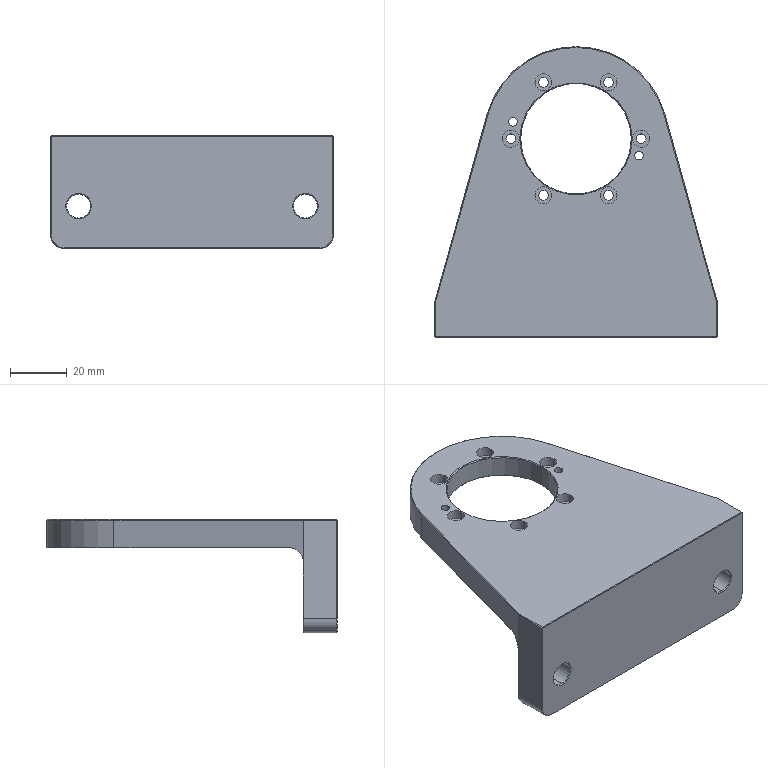NC program | NX | posted with a generic post | part box 100 x 102.5 x 40 mm
Lines 4148 to 4503 of 4503:
(ZLEVEL_PROFILE_COPY_1_COPY_COPY_1 , TOOL : D10JING)
N8264 T14 M6
N8266 G54
N8268 G17 G0 G90 X-58.059 Y-51.322 B0. C0. S9500 M3
N8270 G43 Z30. H14
N8272 Z-19.
N8274 G94 G1 Z-20. F1000.
N8276 X-56.75 Y-50.566
N8278 G3 X-56.25 Y-49.7 R1.
N8280 G1 Y49.7 F1200.
N8282 G2 X-54.786 Y53.236 R5.
N8284 G1 X-54.486 Y53.536
N8286 G2 X-50.95 Y55. R5.
N8288 G1 X-39.25
N8290 G2 X-37.901 Y54.815 R5.
N8292 G1 X28.866 Y36.11
N8294 G2 X28.866 Y-36.11 R37.5
N8296 G1 X-37.901 Y-54.815
N8298 G2 X-39.25 Y-55. R5.
N8300 G1 X-50.95
N8302 G2 X-54.486 Y-53.536 R5.
N8304 G1 X-54.786 Y-53.236
N8306 G2 X-56.25 Y-49.7 R5.
N8308 G3 X-56.75 Y-48.834 R1.
N8310 G1 X-58.25 Y-47.968
N8312 Z-19.
N8314 G0 Z30.
N8316 X-58.059 Y-51.322
N8318 Z-39.
N8320 G1 Z-40. F1000.
N8322 X-56.75 Y-50.566
N8324 G3 X-56.25 Y-49.7 R1.
N8326 G1 Y49.7 F1200.
N8328 G2 X-54.786 Y53.236 R5.
N8330 G1 X-54.486 Y53.536
N8332 G2 X-50.95 Y55. R5.
N8334 G1 X-39.25
N8336 G2 X-37.901 Y54.815 R5.
N8338 G1 X28.866 Y36.11
N8340 G2 X28.866 Y-36.11 R37.5
N8342 G1 X-37.901 Y-54.815
N8344 G2 X-39.25 Y-55. R5.
N8346 G1 X-50.95
N8348 G2 X-54.486 Y-53.536 R5.
N8350 G1 X-54.786 Y-53.236
N8352 G2 X-56.25 Y-49.7 R5.
N8354 G3 X-56.75 Y-48.834 R1.
N8356 G1 X-58.25 Y-47.968
N8358 Z-39.
N8360 G0 Z30.
(ZLEVEL_PROFILE_COPY_1_COPY_COPY_1_COPY , TOOL : D10JING)
N8362 X31.119 Y-1.808
N8364 Z-9.
N8366 G1 Z-10. F1000.
N8368 X32.75 Y-0.866
N8370 G3 X33.25 Y0. R1.
N8372 X18.75 Y14.5 R14.5 F1200.
N8374 X33.25 Y0. R-14.5
N8376 X32.75 Y0.866 R1.
N8378 G1 X31.119 Y1.808
N8380 Z-9.
N8382 G0 Z30.
N8384 M5
(HOLE_MILLING_1 , TOOL : D4)
N8386 T11 M6
N8388 G54
N8390 G17 G0 G90 X-1.169 Y11.5 B0. C0. S9500 M3
N8392 G43 Z30. H11
N8394 Z0.5
N8396 G94 G3 X-1.669 Y11. R0.5 F1350.
N8398 X-1.169 Y10.5 R0.5
N8400 X-1.169 Y10.5 Z0.15 I0. J1.
N8402 X-1.169 Y10.5 Z-0.2 I0. J1.
N8404 X-1.169 Y10.5 Z-0.55 I0. J1.
N8406 X-1.169 Y10.5 Z-0.9 I0. J1.
N8408 X-1.169 Y10.5 Z-1.25 I0. J1.
N8410 X-1.169 Y10.5 Z-1.6 I0. J1.
N8412 X-1.169 Y10.5 Z-1.95 I0. J1.
N8414 X-1.169 Y10.5 Z-2.3 I0. J1.
N8416 X-1.169 Y10.5 Z-2.65 I0. J1.
N8418 X-1.169 Y10.5 Z-3. I0. J1.
N8420 X-1.169 Y10.5 Z-3.35 I0. J1.
N8422 X-0.387 Y10.877 Z-3.4 R1.
N8424 X-0.545 Y12.282 R1.
N8426 X-0.387 Y10.877 R-1.
N8428 X-0.466 Y11.579 R0.5
N8430 X-1.169 Y11.5 R0.5
N8432 G0 Z30.
N8434 X18.75 Y23.
N8436 Z0.5
N8438 G3 X18.25 Y22.5 R0.5
N8440 X18.75 Y22. R0.5
N8442 X18.75 Y22. Z0.15 I0. J1.
N8444 X18.75 Y22. Z-0.2 I0. J1.
N8446 X18.75 Y22. Z-0.55 I0. J1.
N8448 X18.75 Y22. Z-0.9 I0. J1.
N8450 X18.75 Y22. Z-1.25 I0. J1.
N8452 X18.75 Y22. Z-1.6 I0. J1.
N8454 X18.75 Y22. Z-1.95 I0. J1.
N8456 X18.75 Y22. Z-2.3 I0. J1.
N8458 X18.75 Y22. Z-2.65 I0. J1.
N8460 X18.75 Y22. Z-3. I0. J1.
N8462 X18.75 Y22. Z-3.35 I0. J1.
N8464 X19.532 Y22.377 Z-3.4 R1.
N8466 X19.373 Y23.782 R1.
N8468 X19.532 Y22.377 R-1.
N8470 X19.453 Y23.079 R0.5
N8472 X18.75 Y23. R0.5
N8474 G0 Z30.
N8476 X38.669 Y11.5
N8478 Z0.5
N8480 G3 X38.169 Y11. R0.5
N8482 X38.669 Y10.5 R0.5
N8484 X38.669 Y10.5 Z0.15 I0. J1.
N8486 X38.669 Y10.5 Z-0.2 I0. J1.
N8488 X38.669 Y10.5 Z-0.55 I0. J1.
N8490 X38.669 Y10.5 Z-0.9 I0. J1.
N8492 X38.669 Y10.5 Z-1.25 I0. J1.
N8494 X38.669 Y10.5 Z-1.6 I0. J1.
N8496 X38.669 Y10.5 Z-1.95 I0. J1.
N8498 X38.669 Y10.5 Z-2.3 I0. J1.
N8500 X38.669 Y10.5 Z-2.65 I0. J1.
N8502 X38.669 Y10.5 Z-3. I0. J1.
N8504 X38.669 Y10.5 Z-3.35 I0. J1.
N8506 X39.45 Y10.877 Z-3.4 R1.
N8508 X39.292 Y12.282 R1.
N8510 X39.45 Y10.877 R-1.
N8512 X39.371 Y11.579 R0.5
N8514 X38.669 Y11.5 R0.5
N8516 G0 Z30.
N8518 Y-11.5
N8520 Z0.5
N8522 G3 X38.169 Y-12. R0.5
N8524 X38.669 Y-12.5 R0.5
N8526 X38.669 Y-12.5 Z0.15 I0. J1.
N8528 X38.669 Y-12.5 Z-0.2 I0. J1.
N8530 X38.669 Y-12.5 Z-0.55 I0. J1.
N8532 X38.669 Y-12.5 Z-0.9 I0. J1.
N8534 X38.669 Y-12.5 Z-1.25 I0. J1.
N8536 X38.669 Y-12.5 Z-1.6 I0. J1.
N8538 X38.669 Y-12.5 Z-1.95 I0. J1.
N8540 X38.669 Y-12.5 Z-2.3 I0. J1.
N8542 X38.669 Y-12.5 Z-2.65 I0. J1.
N8544 X38.669 Y-12.5 Z-3. I0. J1.
N8546 X38.669 Y-12.5 Z-3.35 I0. J1.
N8548 X39.45 Y-12.123 Z-3.4 R1.
N8550 X39.292 Y-10.718 R1.
N8552 X39.45 Y-12.123 R-1.
N8554 X39.371 Y-11.421 R0.5
N8556 X38.669 Y-11.5 R0.5
N8558 G0 Z30.
N8560 X18.75 Y-23.
N8562 Z0.5
N8564 G3 X18.25 Y-23.5 R0.5
N8566 X18.75 Y-24. R0.5
N8568 X18.75 Y-24. Z0.15 I0. J1.
N8570 X18.75 Y-24. Z-0.2 I0. J1.
N8572 X18.75 Y-24. Z-0.55 I0. J1.
N8574 X18.75 Y-24. Z-0.9 I0. J1.
N8576 X18.75 Y-24. Z-1.25 I0. J1.
N8578 X18.75 Y-24. Z-1.6 I0. J1.
N8580 X18.75 Y-24. Z-1.95 I0. J1.
N8582 X18.75 Y-24. Z-2.3 I0. J1.
N8584 X18.75 Y-24. Z-2.65 I0. J1.
N8586 X18.75 Y-24. Z-3. I0. J1.
N8588 X18.75 Y-24. Z-3.35 I0. J1.
N8590 X19.532 Y-23.623 Z-3.4 R1.
N8592 X19.373 Y-22.218 R1.
N8594 X19.532 Y-23.623 R-1.
N8596 X19.453 Y-22.921 R0.5
N8598 X18.75 Y-23. R0.5
N8600 G0 Z30.
N8602 X-1.169 Y-11.5
N8604 Z0.5
N8606 G3 X-1.669 Y-12. R0.5
N8608 X-1.169 Y-12.5 R0.5
N8610 X-1.169 Y-12.5 Z0.15 I0. J1.
N8612 X-1.169 Y-12.5 Z-0.2 I0. J1.
N8614 X-1.169 Y-12.5 Z-0.55 I0. J1.
N8616 X-1.169 Y-12.5 Z-0.9 I0. J1.
N8618 X-1.169 Y-12.5 Z-1.25 I0. J1.
N8620 X-1.169 Y-12.5 Z-1.6 I0. J1.
N8622 X-1.169 Y-12.5 Z-1.95 I0. J1.
N8624 X-1.169 Y-12.5 Z-2.3 I0. J1.
N8626 X-1.169 Y-12.5 Z-2.65 I0. J1.
N8628 X-1.169 Y-12.5 Z-3. I0. J1.
N8630 X-1.169 Y-12.5 Z-3.35 I0. J1.
N8632 X-0.387 Y-12.123 Z-3.4 R1.
N8634 X-0.545 Y-10.718 R1.
N8636 X-0.387 Y-12.123 R-1.
N8638 X-0.466 Y-11.421 R0.5
N8640 X-1.169 Y-11.5 R0.5
N8642 G0 Z30.
N8644 M5
(PLANAR_MILL_COPY_COPY_COPY_COPY_COPY_COPY_1_COPY_1 , TOOL : D6A45)
N8646 T01 M6
N8648 G54
N8650 G17 G0 G90 X19.616 Y24.7 B0. C0. S9500 M3
N8652 G43 Z30. H1
N8654 Z0.5
N8656 G94 G1 Z-1. F1250.
N8658 G3 X18.75 Y25.2 R1.
N8660 X16.55 Y23. R2.2
N8662 X18.75 Y25.2 R-2.2
N8664 X17.884 Y24.7 R1.
N8666 G1 Z0.5
N8668 G0 Z30.
N8670 X25.153 Y21.783
N8672 Z0.5
N8674 G1 Z-1.
N8676 G3 X25.403 Y22.216 R0.5
N8678 X24.703 Y22.916 R0.7
N8680 X25.403 Y22.216 R-0.7
N8682 X25.153 Y22.649 R0.5
N8684 G1 Z0.5
N8686 G0 Z30.
N8688 X40.369 Y10.634
N8690 Z0.5
N8692 G1 Z-1.
N8694 G3 X40.869 Y11.5 R1.
N8696 X38.669 Y13.7 R2.2
N8698 X40.869 Y11.5 R-2.2
N8700 X40.369 Y12.366 R1.
N8702 G1 Z0.5
N8704 G0 Z30.
N8706 X36.95 Y-0.866
N8708 Z0.5
N8710 G1 Z-1.
N8712 G3 X37.45 Y0. R1.
N8714 X18.75 Y18.7 R18.7
N8716 X37.45 Y0. R-18.7
N8718 X36.95 Y0.866 R1.
N8720 G1 Z0.5
N8722 G0 Z30.
N8724 X40.369 Y-12.366
N8726 Z0.5
N8728 G1 Z-1.
N8730 G3 X40.869 Y-11.5 R1.
N8732 X38.669 Y-9.3 R2.2
N8734 X40.869 Y-11.5 R-2.2
N8736 X40.369 Y-10.634 R1.
N8738 G1 Z0.5
N8740 G0 Z30.
N8742 X17.884 Y-24.7
N8744 Z0.5
N8746 G1 Z-1.
N8748 G3 X18.75 Y-25.2 R1.
N8750 X20.95 Y-23. R2.2
N8752 X18.75 Y-25.2 R-2.2
N8754 X19.616 Y-24.7 R1.
N8756 G1 Z0.5
N8758 G0 Z30.
N8760 X12.364 Y-22.666
N8762 Z0.5
N8764 G1 Z-1.
N8766 G3 X12.797 Y-22.916 R0.5
N8768 X13.497 Y-22.216 R0.7
N8770 X12.797 Y-22.916 R-0.7
N8772 X13.23 Y-22.666 R0.5
N8774 G1 Z0.5
N8776 G0 Z30.
N8778 X-2.035 Y-13.2
N8780 Z0.5
N8782 G1 Z-1.
N8784 G3 X-1.169 Y-13.7 R1.
N8786 X1.031 Y-11.5 R2.2
N8788 X-1.169 Y-13.7 R-2.2
N8790 X-0.303 Y-13.2 R1.
N8792 G1 Z0.5
N8794 G0 Z30.
N8796 X-52.55 Y-0.866
N8798 Z0.5
N8800 G1 Z-1.
N8802 G3 X-52.05 Y0. R1.
N8804 G1 Y49.7
N8806 G2 X-51.816 Y50.266 R0.8
N8808 G1 X-51.516 Y50.566
N8810 G2 X-50.95 Y50.8 R0.8
N8812 G1 X-39.25
N8814 G2 X-39.034 Y50.77 R0.8
N8816 G1 X27.733 Y32.065
N8818 G2 X27.733 Y-32.065 R33.3
N8820 G1 X-39.034 Y-50.77
N8822 G2 X-39.25 Y-50.8 R0.8
N8824 G1 X-50.95
N8826 G2 X-51.516 Y-50.566 R0.8
N8828 G1 X-51.816 Y-50.266
N8830 G2 X-52.05 Y-49.7 R0.8
N8832 G1 Y0.
N8834 G3 X-52.55 Y0.866 R1.
N8836 G1 Z0.5
N8838 G0 Z30.
N8840 X-0.303 Y13.2
N8842 Z0.5
N8844 G1 Z-1.
N8846 G3 X-1.169 Y13.7 R1.
N8848 X-3.369 Y11.5 R2.2
N8850 X-1.169 Y13.7 R-2.2
N8852 X-2.035 Y13.2 R1.
N8854 G1 Z0.5
N8856 G0 Z30.
N8858 M5
(刀补17 , TOOL : D2)
N8860 T17 M6
N8862 G54
N8864 G17 G0 G90 X24.703 Y22.216 B0. C0. S9500 M3
N8866 G43 Z30. H17
N8868 Z0.5
N8870 G41 G94 G1 X24.607 Y22.189 F1000. D17
N8872 G3 X24.703 Y21.766 R0.222
N8874 X24.703 Y21.766 Z-0.5 I0. J0.45
N8876 X24.703 Y21.766 Z-1.5 I0. J0.45
N8878 X24.703 Y21.766 Z-2.5 I0. J0.45
N8880 X24.703 Y21.766 Z-3.5 I0. J0.45
N8882 X24.703 Y21.766 Z-4.5 I0. J0.45
N8884 X24.703 Y21.766 Z-5.5 I0. J0.45
N8886 X24.703 Y21.766 Z-6.5 I0. J0.45
N8888 X24.703 Y21.766 Z-7.5 I0. J0.45
N8890 X24.703 Y22.666 Z-8. I0. J0.45
N8892 X24.253 Y22.216 R0.45
N8894 X24.703 Y22.666 R-0.45
N8896 X24.607 Y22.243 R0.222
N8898 G40
N8900 G1 X24.703 Y22.216
N8902 G0 Z30.
N8904 X12.797 Y-22.216
N8906 Z0.5
N8908 G41 G1 X12.701 Y-22.243
N8910 G3 X12.797 Y-22.666 R0.222
N8912 X12.797 Y-22.666 Z-0.5 I0. J0.45
N8914 X12.797 Y-22.666 Z-1.5 I0. J0.45
N8916 X12.797 Y-22.666 Z-2.5 I0. J0.45
N8918 X12.797 Y-22.666 Z-3.5 I0. J0.45
N8920 X12.797 Y-22.666 Z-4.5 I0. J0.45
N8922 X12.797 Y-22.666 Z-5.5 I0. J0.45
N8924 X12.797 Y-22.666 Z-6.5 I0. J0.45
N8926 X12.797 Y-22.666 Z-7.5 I0. J0.45
N8928 X12.797 Y-21.766 Z-8. I0. J0.45
N8930 X12.347 Y-22.216 R0.45
N8932 X12.797 Y-21.766 R-0.45
N8934 X12.701 Y-22.189 R0.222
N8936 G40
N8938 G1 X12.797 Y-22.216
N8940 G0 Z30.
N8942 M5
N8944 M2